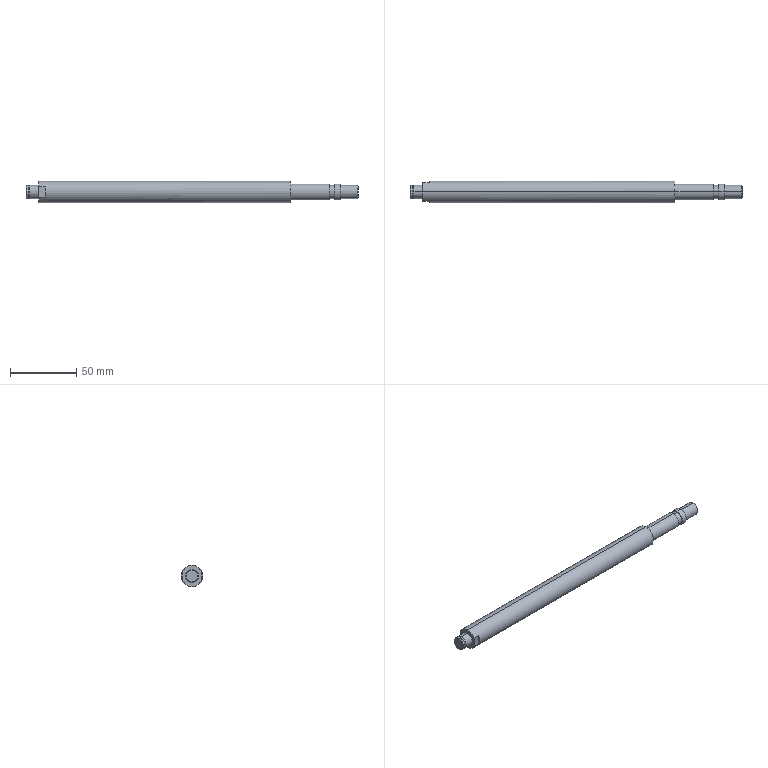Part | SolidWorks | features Chamfer 1, ICE 1, Revolution 1 | 1 solid | 33 faces | box 250 x 16 x 16 mm | volume 43988 mm3 | cylinder 16 | plane 13 | cone 4 | commonest cylinder face diameters 10 x8 12 x4 9.6 x2 16 x2
STEP:
#1=CARTESIAN_POINT('',(250.,0.,-4.5));
#2=VERTEX_POINT('',#1);
#3=CARTESIAN_POINT('',(250.,0.,4.5));
#4=VERTEX_POINT('',#3);
#5=CARTESIAN_POINT('',(250.,0.,0.));
#6=DIRECTION('',(1.,0.,0.));
#7=DIRECTION('',(0.,0.,1.));
#8=AXIS2_PLACEMENT_3D('',#5,#6,#7);
#9=CIRCLE('',#8,4.5);
#10=EDGE_CURVE('',#2,#4,#9,.T.);
#11=ORIENTED_EDGE('',*,*,#10,.F.);
#12=CARTESIAN_POINT('',(249.5,0.,-5.));
#13=VERTEX_POINT('',#12);
#14=CARTESIAN_POINT('',(249.5,0.,-5.));
#15=DIRECTION('',(-0.7071,0.,-0.7071));
#16=VECTOR('',#15,1000.);
#17=LINE('',#14,#16);
#18=EDGE_CURVE('',#2,#13,#17,.T.);
#19=ORIENTED_EDGE('',*,*,#18,.T.);
#20=CARTESIAN_POINT('',(249.5,0.,5.));
#21=VERTEX_POINT('',#20);
#22=CARTESIAN_POINT('',(249.5,0.,0.));
#23=DIRECTION('',(-1.,0.,0.));
#24=DIRECTION('',(0.,0.,1.));
#25=AXIS2_PLACEMENT_3D('',#22,#23,#24);
#26=CIRCLE('',#25,5.);
#27=EDGE_CURVE('',#21,#13,#26,.T.);
#28=ORIENTED_EDGE('',*,*,#27,.F.);
#29=CARTESIAN_POINT('',(249.5,0.,5.));
#30=DIRECTION('',(-0.7071,0.,0.7071));
#31=VECTOR('',#30,1000.);
#32=LINE('',#29,#31);
#33=EDGE_CURVE('',#4,#21,#32,.T.);
#34=ORIENTED_EDGE('',*,*,#33,.F.);
#35=EDGE_LOOP('',(#11,#19,#28,#34));
#36=FACE_OUTER_BOUND('',#35,.T.);
#37=CARTESIAN_POINT('',(249.5,0.,0.));
#38=DIRECTION('',(-1.,0.,0.));
#39=DIRECTION('',(0.,0.,1.));
#40=AXIS2_PLACEMENT_3D('',#37,#38,#39);
#41=CONICAL_SURFACE('',#40,5.,0.7854);
#42=ADVANCED_FACE('',(#36),#41,.T.);
#43=CARTESIAN_POINT('',(0.,0.,4.5));
#44=VERTEX_POINT('',#43);
#45=CARTESIAN_POINT('',(0.,0.,-4.5));
#46=VERTEX_POINT('',#45);
#47=CARTESIAN_POINT('',(0.,0.,0.));
#48=DIRECTION('',(-1.,0.,0.));
#49=DIRECTION('',(0.,0.,-1.));
#50=AXIS2_PLACEMENT_3D('',#47,#48,#49);
#51=CIRCLE('',#50,4.5);
#52=EDGE_CURVE('',#44,#46,#51,.T.);
#53=ORIENTED_EDGE('',*,*,#52,.F.);
#54=CARTESIAN_POINT('',(0.5,0.,5.));
#55=VERTEX_POINT('',#54);
#56=CARTESIAN_POINT('',(0.,0.,4.5));
#57=DIRECTION('',(0.7071,0.,0.7071));
#58=VECTOR('',#57,1000.);
#59=LINE('',#56,#58);
#60=EDGE_CURVE('',#44,#55,#59,.T.);
#61=ORIENTED_EDGE('',*,*,#60,.T.);
#62=CARTESIAN_POINT('',(0.5,0.,-5.));
#63=VERTEX_POINT('',#62);
#64=CARTESIAN_POINT('',(0.5,0.,0.));
#65=DIRECTION('',(1.,0.,0.));
#66=DIRECTION('',(0.,0.,-1.));
#67=AXIS2_PLACEMENT_3D('',#64,#65,#66);
#68=CIRCLE('',#67,5.);
#69=EDGE_CURVE('',#63,#55,#68,.T.);
#70=ORIENTED_EDGE('',*,*,#69,.F.);
#71=CARTESIAN_POINT('',(0.,0.,-4.5));
#72=DIRECTION('',(0.7071,0.,-0.7071));
#73=VECTOR('',#72,1000.);
#74=LINE('',#71,#73);
#75=EDGE_CURVE('',#46,#63,#74,.T.);
#76=ORIENTED_EDGE('',*,*,#75,.F.);
#77=EDGE_LOOP('',(#53,#61,#70,#76));
#78=FACE_OUTER_BOUND('',#77,.T.);
#79=CARTESIAN_POINT('',(0.,0.,0.));
#80=DIRECTION('',(1.,0.,0.));
#81=DIRECTION('',(0.,0.,-1.));
#82=AXIS2_PLACEMENT_3D('',#79,#80,#81);
#83=CONICAL_SURFACE('',#82,4.5,0.7854);
#84=ADVANCED_FACE('',(#78),#83,.T.);
#85=ORIENTED_EDGE('',*,*,#27,.T.);
#86=CARTESIAN_POINT('',(236.5,0.,-5.));
#87=VERTEX_POINT('',#86);
#88=CARTESIAN_POINT('',(0.,0.,-5.));
#89=DIRECTION('',(-1.,0.,0.));
#90=VECTOR('',#89,1000.);
#91=LINE('',#88,#90);
#92=EDGE_CURVE('',#13,#87,#91,.T.);
#93=ORIENTED_EDGE('',*,*,#92,.T.);
#94=CARTESIAN_POINT('',(236.5,0.,5.));
#95=VERTEX_POINT('',#94);
#96=CARTESIAN_POINT('',(236.5,0.,0.));
#97=DIRECTION('',(-1.,0.,0.));
#98=DIRECTION('',(0.,0.,1.));
#99=AXIS2_PLACEMENT_3D('',#96,#97,#98);
#100=CIRCLE('',#99,5.);
#101=EDGE_CURVE('',#95,#87,#100,.T.);
#102=ORIENTED_EDGE('',*,*,#101,.F.);
#103=CARTESIAN_POINT('',(0.,0.,5.));
#104=DIRECTION('',(-1.,0.,0.));
#105=VECTOR('',#104,1000.);
#106=LINE('',#103,#105);
#107=EDGE_CURVE('',#21,#95,#106,.T.);
#108=ORIENTED_EDGE('',*,*,#107,.F.);
#109=EDGE_LOOP('',(#85,#93,#102,#108));
#110=FACE_OUTER_BOUND('',#109,.T.);
#111=CARTESIAN_POINT('',(0.,0.,0.));
#112=DIRECTION('',(-1.,0.,0.));
#113=DIRECTION('',(0.,0.,1.));
#114=AXIS2_PLACEMENT_3D('',#111,#112,#113);
#115=CYLINDRICAL_SURFACE('',#114,5.);
#116=ADVANCED_FACE('',(#110),#115,.T.);
#117=CARTESIAN_POINT('',(236.5,0.,6.));
#118=VERTEX_POINT('',#117);
#119=CARTESIAN_POINT('',(236.5,0.,-6.));
#120=VERTEX_POINT('',#119);
#121=CARTESIAN_POINT('',(236.5,0.,0.));
#122=DIRECTION('',(-1.,0.,0.));
#123=DIRECTION('',(0.,0.,1.));
#124=AXIS2_PLACEMENT_3D('',#121,#122,#123);
#125=CIRCLE('',#124,6.);
#126=EDGE_CURVE('',#118,#120,#125,.T.);
#127=ORIENTED_EDGE('',*,*,#126,.T.);
#128=CARTESIAN_POINT('',(232.5,0.,-6.));
#129=VERTEX_POINT('',#128);
#130=CARTESIAN_POINT('',(0.,0.,-6.));
#131=DIRECTION('',(-1.,0.,0.));
#132=VECTOR('',#131,1000.);
#133=LINE('',#130,#132);
#134=EDGE_CURVE('',#120,#129,#133,.T.);
#135=ORIENTED_EDGE('',*,*,#134,.T.);
#136=CARTESIAN_POINT('',(232.5,0.,6.));
#137=VERTEX_POINT('',#136);
#138=CARTESIAN_POINT('',(232.5,0.,0.));
#139=DIRECTION('',(-1.,0.,0.));
#140=DIRECTION('',(0.,0.,1.));
#141=AXIS2_PLACEMENT_3D('',#138,#139,#140);
#142=CIRCLE('',#141,6.);
#143=EDGE_CURVE('',#137,#129,#142,.T.);
#144=ORIENTED_EDGE('',*,*,#143,.F.);
#145=CARTESIAN_POINT('',(0.,0.,6.));
#146=DIRECTION('',(-1.,0.,0.));
#147=VECTOR('',#146,1000.);
#148=LINE('',#145,#147);
#149=EDGE_CURVE('',#118,#137,#148,.T.);
#150=ORIENTED_EDGE('',*,*,#149,.F.);
#151=EDGE_LOOP('',(#127,#135,#144,#150));
#152=FACE_OUTER_BOUND('',#151,.T.);
#153=CARTESIAN_POINT('',(0.,0.,0.));
#154=DIRECTION('',(-1.,0.,0.));
#155=DIRECTION('',(0.,0.,1.));
#156=AXIS2_PLACEMENT_3D('',#153,#154,#155);
#157=CYLINDRICAL_SURFACE('',#156,6.);
#158=ADVANCED_FACE('',(#152),#157,.T.);
#159=CARTESIAN_POINT('',(232.5,0.,5.));
#160=VERTEX_POINT('',#159);
#161=CARTESIAN_POINT('',(232.5,0.,-5.));
#162=VERTEX_POINT('',#161);
#163=CARTESIAN_POINT('',(232.5,0.,0.));
#164=DIRECTION('',(-1.,0.,0.));
#165=DIRECTION('',(0.,0.,1.));
#166=AXIS2_PLACEMENT_3D('',#163,#164,#165);
#167=CIRCLE('',#166,5.);
#168=EDGE_CURVE('',#160,#162,#167,.T.);
#169=ORIENTED_EDGE('',*,*,#168,.T.);
#170=CARTESIAN_POINT('',(228.5,0.,-5.));
#171=VERTEX_POINT('',#170);
#172=CARTESIAN_POINT('',(0.,0.,-5.));
#173=DIRECTION('',(-1.,0.,0.));
#174=VECTOR('',#173,1000.);
#175=LINE('',#172,#174);
#176=EDGE_CURVE('',#162,#171,#175,.T.);
#177=ORIENTED_EDGE('',*,*,#176,.T.);
#178=CARTESIAN_POINT('',(228.5,0.,5.));
#179=VERTEX_POINT('',#178);
#180=CARTESIAN_POINT('',(228.5,0.,0.));
#181=DIRECTION('',(-1.,0.,0.));
#182=DIRECTION('',(0.,0.,1.));
#183=AXIS2_PLACEMENT_3D('',#180,#181,#182);
#184=CIRCLE('',#183,5.);
#185=EDGE_CURVE('',#179,#171,#184,.T.);
#186=ORIENTED_EDGE('',*,*,#185,.F.);
#187=CARTESIAN_POINT('',(0.,0.,5.));
#188=DIRECTION('',(-1.,0.,0.));
#189=VECTOR('',#188,1000.);
#190=LINE('',#187,#189);
#191=EDGE_CURVE('',#160,#179,#190,.T.);
#192=ORIENTED_EDGE('',*,*,#191,.F.);
#193=EDGE_LOOP('',(#169,#177,#186,#192));
#194=FACE_OUTER_BOUND('',#193,.T.);
#195=CARTESIAN_POINT('',(0.,0.,0.));
#196=DIRECTION('',(-1.,0.,0.));
#197=DIRECTION('',(0.,0.,1.));
#198=AXIS2_PLACEMENT_3D('',#195,#196,#197);
#199=CYLINDRICAL_SURFACE('',#198,5.);
#200=ADVANCED_FACE('',(#194),#199,.T.);
#201=CARTESIAN_POINT('',(228.5,0.,6.));
#202=VERTEX_POINT('',#201);
#203=CARTESIAN_POINT('',(228.5,0.,-6.));
#204=VERTEX_POINT('',#203);
#205=CARTESIAN_POINT('',(228.5,0.,0.));
#206=DIRECTION('',(-1.,0.,0.));
#207=DIRECTION('',(0.,0.,1.));
#208=AXIS2_PLACEMENT_3D('',#205,#206,#207);
#209=CIRCLE('',#208,6.);
#210=EDGE_CURVE('',#202,#204,#209,.T.);
#211=ORIENTED_EDGE('',*,*,#210,.T.);
#212=CARTESIAN_POINT('',(199.5,0.,-6.));
#213=VERTEX_POINT('',#212);
#214=CARTESIAN_POINT('',(0.,0.,-6.));
#215=DIRECTION('',(-1.,0.,0.));
#216=VECTOR('',#215,1000.);
#217=LINE('',#214,#216);
#218=EDGE_CURVE('',#204,#213,#217,.T.);
#219=ORIENTED_EDGE('',*,*,#218,.T.);
#220=CARTESIAN_POINT('',(199.5,0.,6.));
#221=VERTEX_POINT('',#220);
#222=CARTESIAN_POINT('',(199.5,0.,0.));
#223=DIRECTION('',(-1.,0.,0.));
#224=DIRECTION('',(0.,0.,1.));
#225=AXIS2_PLACEMENT_3D('',#222,#223,#224);
#226=CIRCLE('',#225,6.);
#227=EDGE_CURVE('',#221,#213,#226,.T.);
#228=ORIENTED_EDGE('',*,*,#227,.F.);
#229=CARTESIAN_POINT('',(0.,0.,6.));
#230=DIRECTION('',(-1.,0.,0.));
#231=VECTOR('',#230,1000.);
#232=LINE('',#229,#231);
#233=EDGE_CURVE('',#202,#221,#232,.T.);
#234=ORIENTED_EDGE('',*,*,#233,.F.);
#235=EDGE_LOOP('',(#211,#219,#228,#234));
#236=FACE_OUTER_BOUND('',#235,.T.);
#237=CARTESIAN_POINT('',(0.,0.,0.));
#238=DIRECTION('',(-1.,0.,0.));
#239=DIRECTION('',(0.,0.,1.));
#240=AXIS2_PLACEMENT_3D('',#237,#238,#239);
#241=CYLINDRICAL_SURFACE('',#240,6.);
#242=ADVANCED_FACE('',(#236),#241,.T.);
#243=CARTESIAN_POINT('',(9.5,0.,5.));
#244=VERTEX_POINT('',#243);
#245=CARTESIAN_POINT('',(9.5,0.,-5.));
#246=VERTEX_POINT('',#245);
#247=CARTESIAN_POINT('',(9.5,0.,0.));
#248=DIRECTION('',(-1.,0.,0.));
#249=DIRECTION('',(0.,0.,1.));
#250=AXIS2_PLACEMENT_3D('',#247,#248,#249);
#251=CIRCLE('',#250,5.);
#252=EDGE_CURVE('',#244,#246,#251,.T.);
#253=ORIENTED_EDGE('',*,*,#252,.T.);
#254=CARTESIAN_POINT('',(3.,0.,-5.));
#255=VERTEX_POINT('',#254);
#256=CARTESIAN_POINT('',(0.,0.,-5.));
#257=DIRECTION('',(-1.,0.,0.));
#258=VECTOR('',#257,1000.);
#259=LINE('',#256,#258);
#260=EDGE_CURVE('',#246,#255,#259,.T.);
#261=ORIENTED_EDGE('',*,*,#260,.T.);
#262=CARTESIAN_POINT('',(3.,0.,5.));
#263=VERTEX_POINT('',#262);
#264=CARTESIAN_POINT('',(3.,0.,0.));
#265=DIRECTION('',(-1.,0.,0.));
#266=DIRECTION('',(0.,0.,1.));
#267=AXIS2_PLACEMENT_3D('',#264,#265,#266);
#268=CIRCLE('',#267,5.);
#269=EDGE_CURVE('',#263,#255,#268,.T.);
#270=ORIENTED_EDGE('',*,*,#269,.F.);
#271=CARTESIAN_POINT('',(0.,0.,5.));
#272=DIRECTION('',(-1.,0.,0.));
#273=VECTOR('',#272,1000.);
#274=LINE('',#271,#273);
#275=EDGE_CURVE('',#244,#263,#274,.T.);
#276=ORIENTED_EDGE('',*,*,#275,.F.);
#277=EDGE_LOOP('',(#253,#261,#270,#276));
#278=FACE_OUTER_BOUND('',#277,.T.);
#279=CARTESIAN_POINT('',(0.,0.,0.));
#280=DIRECTION('',(-1.,0.,0.));
#281=DIRECTION('',(0.,0.,1.));
#282=AXIS2_PLACEMENT_3D('',#279,#280,#281);
#283=CYLINDRICAL_SURFACE('',#282,5.);
#284=ADVANCED_FACE('',(#278),#283,.T.);
#285=CARTESIAN_POINT('',(3.,0.,4.8));
#286=VERTEX_POINT('',#285);
#287=CARTESIAN_POINT('',(3.,0.,-4.8));
#288=VERTEX_POINT('',#287);
#289=CARTESIAN_POINT('',(3.,0.,0.));
#290=DIRECTION('',(-1.,0.,0.));
#291=DIRECTION('',(0.,0.,1.));
#292=AXIS2_PLACEMENT_3D('',#289,#290,#291);
#293=CIRCLE('',#292,4.8);
#294=EDGE_CURVE('',#286,#288,#293,.T.);
#295=ORIENTED_EDGE('',*,*,#294,.T.);
#296=CARTESIAN_POINT('',(1.85,0.,-4.8));
#297=VERTEX_POINT('',#296);
#298=CARTESIAN_POINT('',(0.,0.,-4.8));
#299=DIRECTION('',(-1.,0.,0.));
#300=VECTOR('',#299,1000.);
#301=LINE('',#298,#300);
#302=EDGE_CURVE('',#288,#297,#301,.T.);
#303=ORIENTED_EDGE('',*,*,#302,.T.);
#304=CARTESIAN_POINT('',(1.85,0.,4.8));
#305=VERTEX_POINT('',#304);
#306=CARTESIAN_POINT('',(1.85,0.,0.));
#307=DIRECTION('',(-1.,0.,0.));
#308=DIRECTION('',(0.,0.,1.));
#309=AXIS2_PLACEMENT_3D('',#306,#307,#308);
#310=CIRCLE('',#309,4.8);
#311=EDGE_CURVE('',#305,#297,#310,.T.);
#312=ORIENTED_EDGE('',*,*,#311,.F.);
#313=CARTESIAN_POINT('',(0.,0.,4.8));
#314=DIRECTION('',(-1.,0.,0.));
#315=VECTOR('',#314,1000.);
#316=LINE('',#313,#315);
#317=EDGE_CURVE('',#286,#305,#316,.T.);
#318=ORIENTED_EDGE('',*,*,#317,.F.);
#319=EDGE_LOOP('',(#295,#303,#312,#318));
#320=FACE_OUTER_BOUND('',#319,.T.);
#321=CARTESIAN_POINT('',(0.,0.,0.));
#322=DIRECTION('',(-1.,0.,0.));
#323=DIRECTION('',(0.,0.,1.));
#324=AXIS2_PLACEMENT_3D('',#321,#322,#323);
#325=CYLINDRICAL_SURFACE('',#324,4.8);
#326=ADVANCED_FACE('',(#320),#325,.T.);
#327=CARTESIAN_POINT('',(1.85,0.,5.));
#328=VERTEX_POINT('',#327);
#329=CARTESIAN_POINT('',(1.85,0.,-5.));
#330=VERTEX_POINT('',#329);
#331=CARTESIAN_POINT('',(1.85,0.,0.));
#332=DIRECTION('',(-1.,0.,0.));
#333=DIRECTION('',(0.,0.,1.));
#334=AXIS2_PLACEMENT_3D('',#331,#332,#333);
#335=CIRCLE('',#334,5.);
#336=EDGE_CURVE('',#328,#330,#335,.T.);
#337=ORIENTED_EDGE('',*,*,#336,.T.);
#338=CARTESIAN_POINT('',(0.,0.,-5.));
#339=DIRECTION('',(-1.,0.,0.));
#340=VECTOR('',#339,1000.);
#341=LINE('',#338,#340);
#342=EDGE_CURVE('',#330,#63,#341,.T.);
#343=ORIENTED_EDGE('',*,*,#342,.T.);
#344=ORIENTED_EDGE('',*,*,#69,.T.);
#345=CARTESIAN_POINT('',(0.,0.,5.));
#346=DIRECTION('',(-1.,0.,0.));
#347=VECTOR('',#346,1000.);
#348=LINE('',#345,#347);
#349=EDGE_CURVE('',#328,#55,#348,.T.);
#350=ORIENTED_EDGE('',*,*,#349,.F.);
#351=EDGE_LOOP('',(#337,#343,#344,#350));
#352=FACE_OUTER_BOUND('',#351,.T.);
#353=CARTESIAN_POINT('',(0.,0.,0.));
#354=DIRECTION('',(-1.,0.,0.));
#355=DIRECTION('',(0.,0.,1.));
#356=AXIS2_PLACEMENT_3D('',#353,#354,#355);
#357=CYLINDRICAL_SURFACE('',#356,5.);
#358=ADVANCED_FACE('',(#352),#357,.T.);
#359=CARTESIAN_POINT('',(199.5,0.,8.));
#360=VERTEX_POINT('',#359);
#361=CARTESIAN_POINT('',(199.5,0.,-8.));
#362=VERTEX_POINT('',#361);
#363=CARTESIAN_POINT('',(199.5,0.,0.));
#364=DIRECTION('',(-1.,0.,0.));
#365=DIRECTION('',(0.,0.,1.));
#366=AXIS2_PLACEMENT_3D('',#363,#364,#365);
#367=CIRCLE('',#366,8.);
#368=EDGE_CURVE('',#360,#362,#367,.T.);
#369=ORIENTED_EDGE('',*,*,#368,.T.);
#370=CARTESIAN_POINT('',(9.5,0.,-8.));
#371=VERTEX_POINT('',#370);
#372=CARTESIAN_POINT('',(0.,0.,-8.));
#373=DIRECTION('',(-1.,0.,0.));
#374=VECTOR('',#373,1000.);
#375=LINE('',#372,#374);
#376=EDGE_CURVE('',#362,#371,#375,.T.);
#377=ORIENTED_EDGE('',*,*,#376,.T.);
#378=CARTESIAN_POINT('',(9.5,7.,-3.873));
#379=VERTEX_POINT('',#378);
#380=CARTESIAN_POINT('',(9.5,0.,0.));
#381=DIRECTION('',(-1.,0.,0.));
#382=DIRECTION('',(0.,0.,1.));
#383=AXIS2_PLACEMENT_3D('',#380,#381,#382);
#384=CIRCLE('',#383,8.);
#385=EDGE_CURVE('',#379,#371,#384,.T.);
#386=ORIENTED_EDGE('',*,*,#385,.F.);
#387=CARTESIAN_POINT('',(14.5,7.,-3.873));
#388=VERTEX_POINT('',#387);
#389=CARTESIAN_POINT('',(0.,7.,-3.873));
#390=DIRECTION('',(-1.,0.,0.));
#391=VECTOR('',#390,1000.);
#392=LINE('',#389,#391);
#393=EDGE_CURVE('',#388,#379,#392,.T.);
#394=ORIENTED_EDGE('',*,*,#393,.F.);
#395=CARTESIAN_POINT('',(14.5,7.,3.873));
#396=VERTEX_POINT('',#395);
#397=CARTESIAN_POINT('',(14.5,0.,0.));
#398=DIRECTION('',(-1.,0.,0.));
#399=DIRECTION('',(0.,0.,1.));
#400=AXIS2_PLACEMENT_3D('',#397,#398,#399);
#401=CIRCLE('',#400,8.);
#402=EDGE_CURVE('',#396,#388,#401,.T.);
#403=ORIENTED_EDGE('',*,*,#402,.F.);
#404=CARTESIAN_POINT('',(9.5,7.,3.873));
#405=VERTEX_POINT('',#404);
#406=CARTESIAN_POINT('',(0.,7.,3.873));
#407=DIRECTION('',(1.,0.,0.));
#408=VECTOR('',#407,1000.);
#409=LINE('',#406,#408);
#410=EDGE_CURVE('',#405,#396,#409,.T.);
#411=ORIENTED_EDGE('',*,*,#410,.F.);
#412=CARTESIAN_POINT('',(9.5,0.,8.));
#413=VERTEX_POINT('',#412);
#414=CARTESIAN_POINT('',(9.5,0.,0.));
#415=DIRECTION('',(-1.,0.,0.));
#416=DIRECTION('',(0.,0.,1.));
#417=AXIS2_PLACEMENT_3D('',#414,#415,#416);
#418=CIRCLE('',#417,8.);
#419=EDGE_CURVE('',#413,#405,#418,.T.);
#420=ORIENTED_EDGE('',*,*,#419,.F.);
#421=CARTESIAN_POINT('',(0.,0.,8.));
#422=DIRECTION('',(-1.,0.,0.));
#423=VECTOR('',#422,1000.);
#424=LINE('',#421,#423);
#425=EDGE_CURVE('',#360,#413,#424,.T.);
#426=ORIENTED_EDGE('',*,*,#425,.F.);
#427=EDGE_LOOP('',(#369,#377,#386,#394,#403,#411,#420,#426));
#428=FACE_OUTER_BOUND('',#427,.T.);
#429=CARTESIAN_POINT('',(0.,0.,0.));
#430=DIRECTION('',(-1.,0.,0.));
#431=DIRECTION('',(0.,0.,1.));
#432=AXIS2_PLACEMENT_3D('',#429,#430,#431);
#433=CYLINDRICAL_SURFACE('',#432,8.);
#434=ADVANCED_FACE('',(#428),#433,.T.);
#435=ORIENTED_EDGE('',*,*,#252,.F.);
#436=CARTESIAN_POINT('',(9.5,0.,0.));
#437=DIRECTION('',(-1.,0.,0.));
#438=DIRECTION('',(0.,0.,1.));
#439=AXIS2_PLACEMENT_3D('',#436,#437,#438);
#440=CIRCLE('',#439,5.);
#441=EDGE_CURVE('',#246,#244,#440,.T.);
#442=ORIENTED_EDGE('',*,*,#441,.F.);
#443=EDGE_LOOP('',(#435,#442));
#444=FACE_BOUND('',#443,.T.);
#445=CARTESIAN_POINT('',(9.5,-7.,-3.873));
#446=VERTEX_POINT('',#445);
#447=CARTESIAN_POINT('',(9.5,-7.,3.873));
#448=VERTEX_POINT('',#447);
#449=CARTESIAN_POINT('',(9.5,-7.,-11.485));
#450=DIRECTION('',(0.,0.,1.));
#451=VECTOR('',#450,1000.);
#452=LINE('',#449,#451);
#453=EDGE_CURVE('',#446,#448,#452,.T.);
#454=ORIENTED_EDGE('',*,*,#453,.T.);
#455=CARTESIAN_POINT('',(9.5,0.,0.));
#456=DIRECTION('',(-1.,0.,0.));
#457=DIRECTION('',(0.,0.,1.));
#458=AXIS2_PLACEMENT_3D('',#455,#456,#457);
#459=CIRCLE('',#458,8.);
#460=EDGE_CURVE('',#448,#413,#459,.T.);
#461=ORIENTED_EDGE('',*,*,#460,.T.);
#462=ORIENTED_EDGE('',*,*,#419,.T.);
#463=CARTESIAN_POINT('',(9.5,7.,-11.485));
#464=DIRECTION('',(0.,0.,-1.));
#465=VECTOR('',#464,1000.);
#466=LINE('',#463,#465);
#467=EDGE_CURVE('',#405,#379,#466,.T.);
#468=ORIENTED_EDGE('',*,*,#467,.T.);
#469=ORIENTED_EDGE('',*,*,#385,.T.);
#470=CARTESIAN_POINT('',(9.5,0.,0.));
#471=DIRECTION('',(-1.,0.,0.));
#472=DIRECTION('',(0.,0.,1.));
#473=AXIS2_PLACEMENT_3D('',#470,#471,#472);
#474=CIRCLE('',#473,8.);
#475=EDGE_CURVE('',#371,#446,#474,.T.);
#476=ORIENTED_EDGE('',*,*,#475,.T.);
#477=EDGE_LOOP('',(#454,#461,#462,#468,#469,#476));
#478=FACE_OUTER_BOUND('',#477,.T.);
#479=CARTESIAN_POINT('',(9.5,5.,0.));
#480=DIRECTION('',(1.,0.,0.));
#481=DIRECTION('',(0.,0.,-1.));
#482=AXIS2_PLACEMENT_3D('',#479,#480,#481);
#483=PLANE('',#482);
#484=ADVANCED_FACE('',(#444,#478),#483,.F.);
#485=ORIENTED_EDGE('',*,*,#376,.F.);
#486=CARTESIAN_POINT('',(199.5,0.,0.));
#487=DIRECTION('',(-1.,0.,0.));
#488=DIRECTION('',(0.,0.,1.));
#489=AXIS2_PLACEMENT_3D('',#486,#487,#488);
#490=CIRCLE('',#489,8.);
#491=EDGE_CURVE('',#362,#360,#490,.T.);
#492=ORIENTED_EDGE('',*,*,#491,.T.);
#493=ORIENTED_EDGE('',*,*,#425,.T.);
#494=ORIENTED_EDGE('',*,*,#460,.F.);
#495=CARTESIAN_POINT('',(14.5,-7.,3.873));
#496=VERTEX_POINT('',#495);
#497=CARTESIAN_POINT('',(0.,-7.,3.873));
#498=DIRECTION('',(-1.,0.,0.));
#499=VECTOR('',#498,1000.);
#500=LINE('',#497,#499);
#501=EDGE_CURVE('',#496,#448,#500,.T.);
#502=ORIENTED_EDGE('',*,*,#501,.F.);
#503=CARTESIAN_POINT('',(14.5,-7.,-3.873));
#504=VERTEX_POINT('',#503);
#505=CARTESIAN_POINT('',(14.5,0.,0.));
#506=DIRECTION('',(-1.,0.,0.));
#507=DIRECTION('',(0.,0.,1.));
#508=AXIS2_PLACEMENT_3D('',#505,#506,#507);
#509=CIRCLE('',#508,8.);
#510=EDGE_CURVE('',#504,#496,#509,.T.);
#511=ORIENTED_EDGE('',*,*,#510,.F.);
#512=CARTESIAN_POINT('',(0.,-7.,-3.873));
#513=DIRECTION('',(1.,0.,0.));
#514=VECTOR('',#513,1000.);
#515=LINE('',#512,#514);
#516=EDGE_CURVE('',#446,#504,#515,.T.);
#517=ORIENTED_EDGE('',*,*,#516,.F.);
#518=ORIENTED_EDGE('',*,*,#475,.F.);
#519=EDGE_LOOP('',(#485,#492,#493,#494,#502,#511,#517,#518));
#520=FACE_OUTER_BOUND('',#519,.T.);
#521=CARTESIAN_POINT('',(0.,0.,0.));
#522=DIRECTION('',(-1.,0.,0.));
#523=DIRECTION('',(0.,0.,1.));
#524=AXIS2_PLACEMENT_3D('',#521,#522,#523);
#525=CYLINDRICAL_SURFACE('',#524,8.);
#526=ADVANCED_FACE('',(#520),#525,.T.);
#527=CARTESIAN_POINT('',(0.,0.,0.));
#528=DIRECTION('',(-1.,0.,0.));
#529=DIRECTION('',(0.,0.,-1.));
#530=AXIS2_PLACEMENT_3D('',#527,#528,#529);
#531=CIRCLE('',#530,4.5);
#532=EDGE_CURVE('',#46,#44,#531,.T.);
#533=ORIENTED_EDGE('',*,*,#532,.T.);
#534=ORIENTED_EDGE('',*,*,#52,.T.);
#535=EDGE_LOOP('',(#533,#534));
#536=FACE_OUTER_BOUND('',#535,.T.);
#537=CARTESIAN_POINT('',(0.,0.,0.));
#538=DIRECTION('',(1.,0.,0.));
#539=DIRECTION('',(0.,0.,-1.));
#540=AXIS2_PLACEMENT_3D('',#537,#538,#539);
#541=PLANE('',#540);
#542=ADVANCED_FACE('',(#536),#541,.F.);
#543=ORIENTED_EDGE('',*,*,#342,.F.);
#544=CARTESIAN_POINT('',(1.85,0.,0.));
#545=DIRECTION('',(-1.,0.,0.));
#546=DIRECTION('',(0.,0.,1.));
#547=AXIS2_PLACEMENT_3D('',#544,#545,#546);
#548=CIRCLE('',#547,5.);
#549=EDGE_CURVE('',#330,#328,#548,.T.);
#550=ORIENTED_EDGE('',*,*,#549,.T.);
#551=ORIENTED_EDGE('',*,*,#349,.T.);
#552=CARTESIAN_POINT('',(0.5,0.,0.));
#553=DIRECTION('',(1.,0.,0.));
#554=DIRECTION('',(0.,0.,-1.));
#555=AXIS2_PLACEMENT_3D('',#552,#553,#554);
#556=CIRCLE('',#555,5.);
#557=EDGE_CURVE('',#55,#63,#556,.T.);
#558=ORIENTED_EDGE('',*,*,#557,.T.);
#559=EDGE_LOOP('',(#543,#550,#551,#558));
#560=FACE_OUTER_BOUND('',#559,.T.);
#561=CARTESIAN_POINT('',(0.,0.,0.));
#562=DIRECTION('',(-1.,0.,0.));
#563=DIRECTION('',(0.,0.,1.));
#564=AXIS2_PLACEMENT_3D('',#561,#562,#563);
#565=CYLINDRICAL_SURFACE('',#564,5.);
#566=ADVANCED_FACE('',(#560),#565,.T.);
#567=ORIENTED_EDGE('',*,*,#336,.F.);
#568=ORIENTED_EDGE('',*,*,#549,.F.);
#569=EDGE_LOOP('',(#567,#568));
#570=FACE_OUTER_BOUND('',#569,.T.);
#571=ORIENTED_EDGE('',*,*,#311,.T.);
#572=CARTESIAN_POINT('',(1.85,0.,0.));
#573=DIRECTION('',(-1.,0.,0.));
#574=DIRECTION('',(0.,0.,1.));
#575=AXIS2_PLACEMENT_3D('',#572,#573,#574);
#576=CIRCLE('',#575,4.8);
#577=EDGE_CURVE('',#297,#305,#576,.T.);
#578=ORIENTED_EDGE('',*,*,#577,.T.);
#579=EDGE_LOOP('',(#571,#578));
#580=FACE_BOUND('',#579,.T.);
#581=CARTESIAN_POINT('',(1.85,5.,0.));
#582=DIRECTION('',(-1.,0.,0.));
#583=DIRECTION('',(0.,0.,1.));
#584=AXIS2_PLACEMENT_3D('',#581,#582,#583);
#585=PLANE('',#584);
#586=ADVANCED_FACE('',(#570,#580),#585,.F.);
#587=ORIENTED_EDGE('',*,*,#302,.F.);
#588=CARTESIAN_POINT('',(3.,0.,0.));
#589=DIRECTION('',(-1.,0.,0.));
#590=DIRECTION('',(0.,0.,1.));
#591=AXIS2_PLACEMENT_3D('',#588,#589,#590);
#592=CIRCLE('',#591,4.8);
#593=EDGE_CURVE('',#288,#286,#592,.T.);
#594=ORIENTED_EDGE('',*,*,#593,.T.);
#595=ORIENTED_EDGE('',*,*,#317,.T.);
#596=ORIENTED_EDGE('',*,*,#577,.F.);
#597=EDGE_LOOP('',(#587,#594,#595,#596));
#598=FACE_OUTER_BOUND('',#597,.T.);
#599=CARTESIAN_POINT('',(0.,0.,0.));
#600=DIRECTION('',(-1.,0.,0.));
#601=DIRECTION('',(0.,0.,1.));
#602=AXIS2_PLACEMENT_3D('',#599,#600,#601);
#603=CYLINDRICAL_SURFACE('',#602,4.8);
#604=ADVANCED_FACE('',(#598),#603,.T.);
#605=ORIENTED_EDGE('',*,*,#294,.F.);
#606=ORIENTED_EDGE('',*,*,#593,.F.);
#607=EDGE_LOOP('',(#605,#606));
#608=FACE_BOUND('',#607,.T.);
#609=ORIENTED_EDGE('',*,*,#269,.T.);
#610=CARTESIAN_POINT('',(3.,0.,0.));
#611=DIRECTION('',(-1.,0.,0.));
#612=DIRECTION('',(0.,0.,1.));
#613=AXIS2_PLACEMENT_3D('',#610,#611,#612);
#614=CIRCLE('',#613,5.);
#615=EDGE_CURVE('',#255,#263,#614,.T.);
#616=ORIENTED_EDGE('',*,*,#615,.T.);
#617=EDGE_LOOP('',(#609,#616));
#618=FACE_OUTER_BOUND('',#617,.T.);
#619=CARTESIAN_POINT('',(3.,4.8,0.));
#620=DIRECTION('',(1.,0.,0.));
#621=DIRECTION('',(0.,0.,-1.));
#622=AXIS2_PLACEMENT_3D('',#619,#620,#621);
#623=PLANE('',#622);
#624=ADVANCED_FACE('',(#608,#618),#623,.F.);
#625=ORIENTED_EDGE('',*,*,#260,.F.);
#626=ORIENTED_EDGE('',*,*,#441,.T.);
#627=ORIENTED_EDGE('',*,*,#275,.T.);
#628=ORIENTED_EDGE('',*,*,#615,.F.);
#629=EDGE_LOOP('',(#625,#626,#627,#628));
#630=FACE_OUTER_BOUND('',#629,.T.);
#631=CARTESIAN_POINT('',(0.,0.,0.));
#632=DIRECTION('',(-1.,0.,0.));
#633=DIRECTION('',(0.,0.,1.));
#634=AXIS2_PLACEMENT_3D('',#631,#632,#633);
#635=CYLINDRICAL_SURFACE('',#634,5.);
#636=ADVANCED_FACE('',(#630),#635,.T.);
#637=ORIENTED_EDGE('',*,*,#368,.F.);
#638=ORIENTED_EDGE('',*,*,#491,.F.);
#639=EDGE_LOOP('',(#637,#638));
#640=FACE_OUTER_BOUND('',#639,.T.);
#641=ORIENTED_EDGE('',*,*,#227,.T.);
#642=CARTESIAN_POINT('',(199.5,0.,0.));
#643=DIRECTION('',(-1.,0.,0.));
#644=DIRECTION('',(0.,0.,1.));
#645=AXIS2_PLACEMENT_3D('',#642,#643,#644);
#646=CIRCLE('',#645,6.);
#647=EDGE_CURVE('',#213,#221,#646,.T.);
#648=ORIENTED_EDGE('',*,*,#647,.T.);
#649=EDGE_LOOP('',(#641,#648));
#650=FACE_BOUND('',#649,.T.);
#651=CARTESIAN_POINT('',(199.5,8.,0.));
#652=DIRECTION('',(-1.,0.,0.));
#653=DIRECTION('',(0.,0.,1.));
#654=AXIS2_PLACEMENT_3D('',#651,#652,#653);
#655=PLANE('',#654);
#656=ADVANCED_FACE('',(#640,#650),#655,.F.);
#657=ORIENTED_EDGE('',*,*,#218,.F.);
#658=CARTESIAN_POINT('',(228.5,0.,0.));
#659=DIRECTION('',(-1.,0.,0.));
#660=DIRECTION('',(0.,0.,1.));
#661=AXIS2_PLACEMENT_3D('',#658,#659,#660);
#662=CIRCLE('',#661,6.);
#663=EDGE_CURVE('',#204,#202,#662,.T.);
#664=ORIENTED_EDGE('',*,*,#663,.T.);
#665=ORIENTED_EDGE('',*,*,#233,.T.);
#666=ORIENTED_EDGE('',*,*,#647,.F.);
#667=EDGE_LOOP('',(#657,#664,#665,#666));
#668=FACE_OUTER_BOUND('',#667,.T.);
#669=CARTESIAN_POINT('',(0.,0.,0.));
#670=DIRECTION('',(-1.,0.,0.));
#671=DIRECTION('',(0.,0.,1.));
#672=AXIS2_PLACEMENT_3D('',#669,#670,#671);
#673=CYLINDRICAL_SURFACE('',#672,6.);
#674=ADVANCED_FACE('',(#668),#673,.T.);
#675=ORIENTED_EDGE('',*,*,#210,.F.);
#676=ORIENTED_EDGE('',*,*,#663,.F.);
#677=EDGE_LOOP('',(#675,#676));
#678=FACE_OUTER_BOUND('',#677,.T.);
#679=ORIENTED_EDGE('',*,*,#185,.T.);
#680=CARTESIAN_POINT('',(228.5,0.,0.));
#681=DIRECTION('',(-1.,0.,0.));
#682=DIRECTION('',(0.,0.,1.));
#683=AXIS2_PLACEMENT_3D('',#680,#681,#682);
#684=CIRCLE('',#683,5.);
#685=EDGE_CURVE('',#171,#179,#684,.T.);
#686=ORIENTED_EDGE('',*,*,#685,.T.);
#687=EDGE_LOOP('',(#679,#686));
#688=FACE_BOUND('',#687,.T.);
#689=CARTESIAN_POINT('',(228.5,6.,0.));
#690=DIRECTION('',(-1.,0.,0.));
#691=DIRECTION('',(0.,0.,1.));
#692=AXIS2_PLACEMENT_3D('',#689,#690,#691);
#693=PLANE('',#692);
#694=ADVANCED_FACE('',(#678,#688),#693,.F.);
#695=ORIENTED_EDGE('',*,*,#176,.F.);
#696=CARTESIAN_POINT('',(232.5,0.,0.));
#697=DIRECTION('',(-1.,0.,0.));
#698=DIRECTION('',(0.,0.,1.));
#699=AXIS2_PLACEMENT_3D('',#696,#697,#698);
#700=CIRCLE('',#699,5.);
#701=EDGE_CURVE('',#162,#160,#700,.T.);
#702=ORIENTED_EDGE('',*,*,#701,.T.);
#703=ORIENTED_EDGE('',*,*,#191,.T.);
#704=ORIENTED_EDGE('',*,*,#685,.F.);
#705=EDGE_LOOP('',(#695,#702,#703,#704));
#706=FACE_OUTER_BOUND('',#705,.T.);
#707=CARTESIAN_POINT('',(0.,0.,0.));
#708=DIRECTION('',(-1.,0.,0.));
#709=DIRECTION('',(0.,0.,1.));
#710=AXIS2_PLACEMENT_3D('',#707,#708,#709);
#711=CYLINDRICAL_SURFACE('',#710,5.);
#712=ADVANCED_FACE('',(#706),#711,.T.);
#713=ORIENTED_EDGE('',*,*,#168,.F.);
#714=ORIENTED_EDGE('',*,*,#701,.F.);
#715=EDGE_LOOP('',(#713,#714));
#716=FACE_BOUND('',#715,.T.);
#717=ORIENTED_EDGE('',*,*,#143,.T.);
#718=CARTESIAN_POINT('',(232.5,0.,0.));
#719=DIRECTION('',(-1.,0.,0.));
#720=DIRECTION('',(0.,0.,1.));
#721=AXIS2_PLACEMENT_3D('',#718,#719,#720);
#722=CIRCLE('',#721,6.);
#723=EDGE_CURVE('',#129,#137,#722,.T.);
#724=ORIENTED_EDGE('',*,*,#723,.T.);
#725=EDGE_LOOP('',(#717,#724));
#726=FACE_OUTER_BOUND('',#725,.T.);
#727=CARTESIAN_POINT('',(232.5,5.,0.));
#728=DIRECTION('',(1.,0.,0.));
#729=DIRECTION('',(0.,0.,-1.));
#730=AXIS2_PLACEMENT_3D('',#727,#728,#729);
#731=PLANE('',#730);
#732=ADVANCED_FACE('',(#716,#726),#731,.F.);
#733=ORIENTED_EDGE('',*,*,#134,.F.);
#734=CARTESIAN_POINT('',(236.5,0.,0.));
#735=DIRECTION('',(-1.,0.,0.));
#736=DIRECTION('',(0.,0.,1.));
#737=AXIS2_PLACEMENT_3D('',#734,#735,#736);
#738=CIRCLE('',#737,6.);
#739=EDGE_CURVE('',#120,#118,#738,.T.);
#740=ORIENTED_EDGE('',*,*,#739,.T.);
#741=ORIENTED_EDGE('',*,*,#149,.T.);
#742=ORIENTED_EDGE('',*,*,#723,.F.);
#743=EDGE_LOOP('',(#733,#740,#741,#742));
#744=FACE_OUTER_BOUND('',#743,.T.);
#745=CARTESIAN_POINT('',(0.,0.,0.));
#746=DIRECTION('',(-1.,0.,0.));
#747=DIRECTION('',(0.,0.,1.));
#748=AXIS2_PLACEMENT_3D('',#745,#746,#747);
#749=CYLINDRICAL_SURFACE('',#748,6.);
#750=ADVANCED_FACE('',(#744),#749,.T.);
#751=ORIENTED_EDGE('',*,*,#126,.F.);
#752=ORIENTED_EDGE('',*,*,#739,.F.);
#753=EDGE_LOOP('',(#751,#752));
#754=FACE_OUTER_BOUND('',#753,.T.);
#755=ORIENTED_EDGE('',*,*,#101,.T.);
#756=CARTESIAN_POINT('',(236.5,0.,0.));
#757=DIRECTION('',(-1.,0.,0.));
#758=DIRECTION('',(0.,0.,1.));
#759=AXIS2_PLACEMENT_3D('',#756,#757,#758);
#760=CIRCLE('',#759,5.);
#761=EDGE_CURVE('',#87,#95,#760,.T.);
#762=ORIENTED_EDGE('',*,*,#761,.T.);
#763=EDGE_LOOP('',(#755,#762));
#764=FACE_BOUND('',#763,.T.);
#765=CARTESIAN_POINT('',(236.5,6.,0.));
#766=DIRECTION('',(-1.,0.,0.));
#767=DIRECTION('',(0.,0.,1.));
#768=AXIS2_PLACEMENT_3D('',#765,#766,#767);
#769=PLANE('',#768);
#770=ADVANCED_FACE('',(#754,#764),#769,.F.);
#771=ORIENTED_EDGE('',*,*,#92,.F.);
#772=CARTESIAN_POINT('',(249.5,0.,0.));
#773=DIRECTION('',(-1.,0.,0.));
#774=DIRECTION('',(0.,0.,1.));
#775=AXIS2_PLACEMENT_3D('',#772,#773,#774);
#776=CIRCLE('',#775,5.);
#777=EDGE_CURVE('',#13,#21,#776,.T.);
#778=ORIENTED_EDGE('',*,*,#777,.T.);
#779=ORIENTED_EDGE('',*,*,#107,.T.);
#780=ORIENTED_EDGE('',*,*,#761,.F.);
#781=EDGE_LOOP('',(#771,#778,#779,#780));
#782=FACE_OUTER_BOUND('',#781,.T.);
#783=CARTESIAN_POINT('',(0.,0.,0.));
#784=DIRECTION('',(-1.,0.,0.));
#785=DIRECTION('',(0.,0.,1.));
#786=AXIS2_PLACEMENT_3D('',#783,#784,#785);
#787=CYLINDRICAL_SURFACE('',#786,5.);
#788=ADVANCED_FACE('',(#782),#787,.T.);
#789=CARTESIAN_POINT('',(250.,0.,0.));
#790=DIRECTION('',(1.,0.,0.));
#791=DIRECTION('',(0.,0.,1.));
#792=AXIS2_PLACEMENT_3D('',#789,#790,#791);
#793=CIRCLE('',#792,4.5);
#794=EDGE_CURVE('',#4,#2,#793,.T.);
#795=ORIENTED_EDGE('',*,*,#794,.T.);
#796=ORIENTED_EDGE('',*,*,#10,.T.);
#797=EDGE_LOOP('',(#795,#796));
#798=FACE_OUTER_BOUND('',#797,.T.);
#799=CARTESIAN_POINT('',(250.,5.,0.));
#800=DIRECTION('',(-1.,0.,0.));
#801=DIRECTION('',(0.,0.,1.));
#802=AXIS2_PLACEMENT_3D('',#799,#800,#801);
#803=PLANE('',#802);
#804=ADVANCED_FACE('',(#798),#803,.F.);
#805=ORIENTED_EDGE('',*,*,#393,.T.);
#806=ORIENTED_EDGE('',*,*,#467,.F.);
#807=ORIENTED_EDGE('',*,*,#410,.T.);
#808=CARTESIAN_POINT('',(14.5,7.,-11.485));
#809=DIRECTION('',(0.,0.,-1.));
#810=VECTOR('',#809,1000.);
#811=LINE('',#808,#810);
#812=EDGE_CURVE('',#396,#388,#811,.T.);
#813=ORIENTED_EDGE('',*,*,#812,.T.);
#814=EDGE_LOOP('',(#805,#806,#807,#813));
#815=FACE_OUTER_BOUND('',#814,.T.);
#816=CARTESIAN_POINT('',(14.5,7.,-11.485));
#817=DIRECTION('',(0.,1.,0.));
#818=DIRECTION('',(0.,0.,1.));
#819=AXIS2_PLACEMENT_3D('',#816,#817,#818);
#820=PLANE('',#819);
#821=ADVANCED_FACE('',(#815),#820,.T.);
#822=ORIENTED_EDGE('',*,*,#402,.T.);
#823=ORIENTED_EDGE('',*,*,#812,.F.);
#824=EDGE_LOOP('',(#822,#823));
#825=FACE_OUTER_BOUND('',#824,.T.);
#826=CARTESIAN_POINT('',(14.5,0.,0.));
#827=DIRECTION('',(-1.,0.,0.));
#828=DIRECTION('',(0.,0.,1.));
#829=AXIS2_PLACEMENT_3D('',#826,#827,#828);
#830=PLANE('',#829);
#831=ADVANCED_FACE('',(#825),#830,.T.);
#832=ORIENTED_EDGE('',*,*,#510,.T.);
#833=CARTESIAN_POINT('',(14.5,-7.,-11.485));
#834=DIRECTION('',(0.,0.,1.));
#835=VECTOR('',#834,1000.);
#836=LINE('',#833,#835);
#837=EDGE_CURVE('',#504,#496,#836,.T.);
#838=ORIENTED_EDGE('',*,*,#837,.F.);
#839=EDGE_LOOP('',(#832,#838));
#840=FACE_OUTER_BOUND('',#839,.T.);
#841=CARTESIAN_POINT('',(14.5,0.,0.));
#842=DIRECTION('',(-1.,0.,0.));
#843=DIRECTION('',(0.,0.,1.));
#844=AXIS2_PLACEMENT_3D('',#841,#842,#843);
#845=PLANE('',#844);
#846=ADVANCED_FACE('',(#840),#845,.T.);
#847=ORIENTED_EDGE('',*,*,#501,.T.);
#848=ORIENTED_EDGE('',*,*,#453,.F.);
#849=ORIENTED_EDGE('',*,*,#516,.T.);
#850=ORIENTED_EDGE('',*,*,#837,.T.);
#851=EDGE_LOOP('',(#847,#848,#849,#850));
#852=FACE_OUTER_BOUND('',#851,.T.);
#853=CARTESIAN_POINT('',(14.5,-7.,-11.485));
#854=DIRECTION('',(0.,-1.,0.));
#855=DIRECTION('',(0.,0.,-1.));
#856=AXIS2_PLACEMENT_3D('',#853,#854,#855);
#857=PLANE('',#856);
#858=ADVANCED_FACE('',(#852),#857,.T.);
#859=ORIENTED_EDGE('',*,*,#60,.F.);
#860=ORIENTED_EDGE('',*,*,#532,.F.);
#861=ORIENTED_EDGE('',*,*,#75,.T.);
#862=ORIENTED_EDGE('',*,*,#557,.F.);
#863=EDGE_LOOP('',(#859,#860,#861,#862));
#864=FACE_OUTER_BOUND('',#863,.T.);
#865=CARTESIAN_POINT('',(0.,0.,0.));
#866=DIRECTION('',(1.,0.,0.));
#867=DIRECTION('',(0.,0.,-1.));
#868=AXIS2_PLACEMENT_3D('',#865,#866,#867);
#869=CONICAL_SURFACE('',#868,4.5,0.7854);
#870=ADVANCED_FACE('',(#864),#869,.T.);
#871=ORIENTED_EDGE('',*,*,#18,.F.);
#872=ORIENTED_EDGE('',*,*,#794,.F.);
#873=ORIENTED_EDGE('',*,*,#33,.T.);
#874=ORIENTED_EDGE('',*,*,#777,.F.);
#875=EDGE_LOOP('',(#871,#872,#873,#874));
#876=FACE_OUTER_BOUND('',#875,.T.);
#877=CARTESIAN_POINT('',(249.5,0.,0.));
#878=DIRECTION('',(-1.,0.,0.));
#879=DIRECTION('',(0.,0.,1.));
#880=AXIS2_PLACEMENT_3D('',#877,#878,#879);
#881=CONICAL_SURFACE('',#880,5.,0.7854);
#882=ADVANCED_FACE('',(#876),#881,.T.);
#883=CLOSED_SHELL('',(#42,#84,#116,#158,#200,#242,#284,#326,#358,#434,#484,#526,#542,#566,#586,#604,#624,#636,#656,#674,#694,#712,#732,#750,#770,#788,#804,#821,#831,#846,#858,#870,#882));
#884=MANIFOLD_SOLID_BREP('',#883);
#885=CARTESIAN_POINT('',(0.,0.,0.));
#886=DIRECTION('',(0.,0.,1.));
#887=DIRECTION('',(1.,0.,0.));
#888=AXIS2_PLACEMENT_3D('',#885,#886,#887);
#889=(LENGTH_UNIT()NAMED_UNIT(*)SI_UNIT(.MILLI.,.METRE.));
#890=UNCERTAINTY_MEASURE_WITH_UNIT(LENGTH_MEASURE(0.00001),#889,'','');
#891=(NAMED_UNIT(*)PLANE_ANGLE_UNIT()SI_UNIT($,.RADIAN.));
#892=(NAMED_UNIT(*)SI_UNIT($,.STERADIAN.)SOLID_ANGLE_UNIT());
#893=(GEOMETRIC_REPRESENTATION_CONTEXT(3)GLOBAL_UNCERTAINTY_ASSIGNED_CONTEXT((#890))GLOBAL_UNIT_ASSIGNED_CONTEXT((#889,#891,#892))REPRESENTATION_CONTEXT('',''));
#894=ADVANCED_BREP_SHAPE_REPRESENTATION('',(#884,#888),#893);